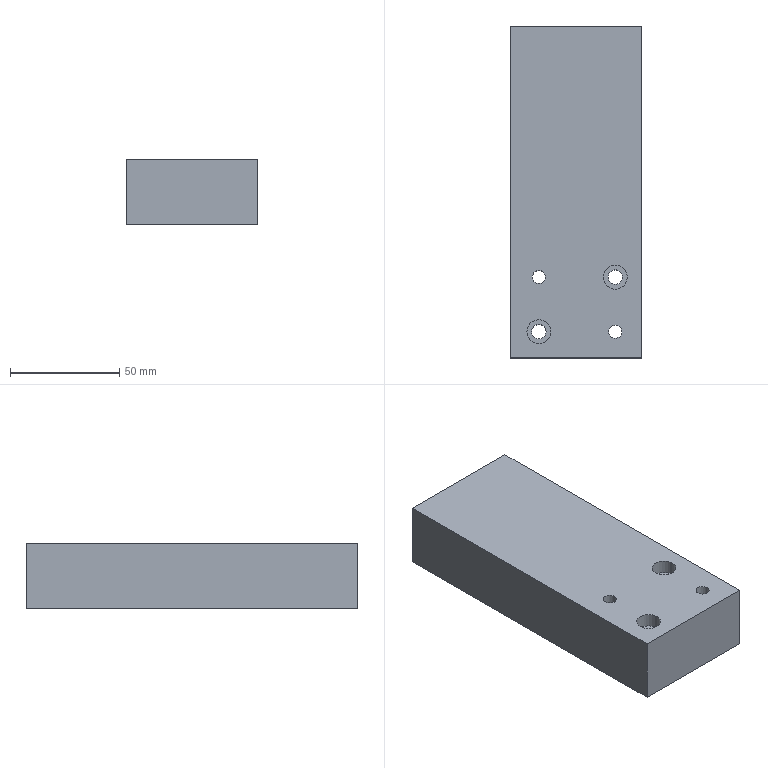Part | NX | features BREP 1 | 1 solid | 22 faces | box 60 x 152 x 30 mm | volume 267751 mm3 | cylinder 10 | plane 8 | cone 4 | commonest cylinder face diameters 6 x4 5 x2 6.6 x2 11 x2
STEP:
#1=CARTESIAN_POINT('',(30.,-76.,0.));
#2=VERTEX_POINT('',#1);
#3=CARTESIAN_POINT('',(30.,76.,0.));
#4=VERTEX_POINT('',#3);
#5=CARTESIAN_POINT('',(30.,76.,0.));
#6=DIRECTION('',(0.,1.,0.));
#7=VECTOR('',#6,1000.);
#8=LINE('',#5,#7);
#9=EDGE_CURVE('',#2,#4,#8,.T.);
#10=ORIENTED_EDGE('',*,*,#9,.T.);
#11=CARTESIAN_POINT('',(30.,76.,30.));
#12=VERTEX_POINT('',#11);
#13=CARTESIAN_POINT('',(30.,76.,30.));
#14=DIRECTION('',(0.,0.,-1.));
#15=VECTOR('',#14,1000.);
#16=LINE('',#13,#15);
#17=EDGE_CURVE('',#12,#4,#16,.T.);
#18=ORIENTED_EDGE('',*,*,#17,.F.);
#19=CARTESIAN_POINT('',(30.,-76.,30.));
#20=VERTEX_POINT('',#19);
#21=CARTESIAN_POINT('',(30.,76.,30.));
#22=DIRECTION('',(0.,1.,0.));
#23=VECTOR('',#22,1000.);
#24=LINE('',#21,#23);
#25=EDGE_CURVE('',#20,#12,#24,.T.);
#26=ORIENTED_EDGE('',*,*,#25,.F.);
#27=CARTESIAN_POINT('',(30.,-76.,30.));
#28=DIRECTION('',(0.,0.,-1.));
#29=VECTOR('',#28,1000.);
#30=LINE('',#27,#29);
#31=EDGE_CURVE('',#20,#2,#30,.T.);
#32=ORIENTED_EDGE('',*,*,#31,.T.);
#33=EDGE_LOOP('',(#10,#18,#26,#32));
#34=FACE_BOUND('',#33,.T.);
#35=CARTESIAN_POINT('',(30.,76.,30.));
#36=DIRECTION('',(-1.,0.,0.));
#37=DIRECTION('',(0.,1.,0.));
#38=AXIS2_PLACEMENT_3D('',#35,#36,#37);
#39=PLANE('',#38);
#40=ADVANCED_FACE('',(#34),#39,.F.);
#41=CARTESIAN_POINT('',(-10.,76.,17.5));
#42=VERTEX_POINT('',#41);
#43=CARTESIAN_POINT('',(-10.,76.,15.));
#44=DIRECTION('',(0.,1.,0.));
#45=DIRECTION('',(0.,0.,1.));
#46=AXIS2_PLACEMENT_3D('',#43,#44,#45);
#47=CIRCLE('',#46,2.5);
#48=EDGE_CURVE('',#42,#42,#47,.T.);
#49=ORIENTED_EDGE('',*,*,#48,.F.);
#50=EDGE_LOOP('',(#49));
#51=FACE_BOUND('',#50,.T.);
#52=CARTESIAN_POINT('',(10.,76.,17.5));
#53=VERTEX_POINT('',#52);
#54=CARTESIAN_POINT('',(10.,76.,15.));
#55=DIRECTION('',(0.,1.,0.));
#56=DIRECTION('',(0.,0.,1.));
#57=AXIS2_PLACEMENT_3D('',#54,#55,#56);
#58=CIRCLE('',#57,2.5);
#59=EDGE_CURVE('',#53,#53,#58,.T.);
#60=ORIENTED_EDGE('',*,*,#59,.F.);
#61=EDGE_LOOP('',(#60));
#62=FACE_BOUND('',#61,.T.);
#63=CARTESIAN_POINT('',(-23.,76.,18.));
#64=VERTEX_POINT('',#63);
#65=CARTESIAN_POINT('',(-23.,76.,15.));
#66=DIRECTION('',(0.,1.,0.));
#67=DIRECTION('',(0.,0.,1.));
#68=AXIS2_PLACEMENT_3D('',#65,#66,#67);
#69=CIRCLE('',#68,3.);
#70=EDGE_CURVE('',#64,#64,#69,.T.);
#71=ORIENTED_EDGE('',*,*,#70,.F.);
#72=EDGE_LOOP('',(#71));
#73=FACE_BOUND('',#72,.T.);
#74=CARTESIAN_POINT('',(23.,76.,18.));
#75=VERTEX_POINT('',#74);
#76=CARTESIAN_POINT('',(23.,76.,15.));
#77=DIRECTION('',(0.,1.,0.));
#78=DIRECTION('',(0.,0.,1.));
#79=AXIS2_PLACEMENT_3D('',#76,#77,#78);
#80=CIRCLE('',#79,3.);
#81=EDGE_CURVE('',#75,#75,#80,.T.);
#82=ORIENTED_EDGE('',*,*,#81,.F.);
#83=EDGE_LOOP('',(#82));
#84=FACE_BOUND('',#83,.T.);
#85=CARTESIAN_POINT('',(-30.,76.,0.));
#86=VERTEX_POINT('',#85);
#87=CARTESIAN_POINT('',(-30.,76.,0.));
#88=DIRECTION('',(-1.,0.,0.));
#89=VECTOR('',#88,1000.);
#90=LINE('',#87,#89);
#91=EDGE_CURVE('',#4,#86,#90,.T.);
#92=ORIENTED_EDGE('',*,*,#91,.T.);
#93=CARTESIAN_POINT('',(-30.,76.,30.));
#94=VERTEX_POINT('',#93);
#95=CARTESIAN_POINT('',(-30.,76.,30.));
#96=DIRECTION('',(0.,0.,-1.));
#97=VECTOR('',#96,1000.);
#98=LINE('',#95,#97);
#99=EDGE_CURVE('',#94,#86,#98,.T.);
#100=ORIENTED_EDGE('',*,*,#99,.F.);
#101=CARTESIAN_POINT('',(-30.,76.,30.));
#102=DIRECTION('',(-1.,0.,0.));
#103=VECTOR('',#102,1000.);
#104=LINE('',#101,#103);
#105=EDGE_CURVE('',#12,#94,#104,.T.);
#106=ORIENTED_EDGE('',*,*,#105,.F.);
#107=ORIENTED_EDGE('',*,*,#17,.T.);
#108=EDGE_LOOP('',(#92,#100,#106,#107));
#109=FACE_BOUND('',#108,.T.);
#110=CARTESIAN_POINT('',(-30.,76.,30.));
#111=DIRECTION('',(0.,-1.,0.));
#112=DIRECTION('',(0.,0.,1.));
#113=AXIS2_PLACEMENT_3D('',#110,#111,#112);
#114=PLANE('',#113);
#115=ADVANCED_FACE('',(#51,#62,#73,#84,#109),#114,.F.);
#116=CARTESIAN_POINT('',(-30.,-76.,0.));
#117=VERTEX_POINT('',#116);
#118=CARTESIAN_POINT('',(-30.,76.,0.));
#119=DIRECTION('',(0.,-1.,0.));
#120=VECTOR('',#119,1000.);
#121=LINE('',#118,#120);
#122=EDGE_CURVE('',#86,#117,#121,.T.);
#123=ORIENTED_EDGE('',*,*,#122,.T.);
#124=CARTESIAN_POINT('',(-30.,-76.,30.));
#125=VERTEX_POINT('',#124);
#126=CARTESIAN_POINT('',(-30.,-76.,30.));
#127=DIRECTION('',(0.,0.,-1.));
#128=VECTOR('',#127,1000.);
#129=LINE('',#126,#128);
#130=EDGE_CURVE('',#125,#117,#129,.T.);
#131=ORIENTED_EDGE('',*,*,#130,.F.);
#132=CARTESIAN_POINT('',(-30.,76.,30.));
#133=DIRECTION('',(0.,-1.,0.));
#134=VECTOR('',#133,1000.);
#135=LINE('',#132,#134);
#136=EDGE_CURVE('',#94,#125,#135,.T.);
#137=ORIENTED_EDGE('',*,*,#136,.F.);
#138=ORIENTED_EDGE('',*,*,#99,.T.);
#139=EDGE_LOOP('',(#123,#131,#137,#138));
#140=FACE_BOUND('',#139,.T.);
#141=CARTESIAN_POINT('',(-30.,76.,30.));
#142=DIRECTION('',(1.,0.,0.));
#143=DIRECTION('',(0.,-1.,0.));
#144=AXIS2_PLACEMENT_3D('',#141,#142,#143);
#145=PLANE('',#144);
#146=ADVANCED_FACE('',(#140),#145,.F.);
#147=CARTESIAN_POINT('',(-30.,-76.,0.));
#148=DIRECTION('',(1.,0.,0.));
#149=VECTOR('',#148,1000.);
#150=LINE('',#147,#149);
#151=EDGE_CURVE('',#117,#2,#150,.T.);
#152=ORIENTED_EDGE('',*,*,#151,.T.);
#153=ORIENTED_EDGE('',*,*,#31,.F.);
#154=CARTESIAN_POINT('',(-30.,-76.,30.));
#155=DIRECTION('',(1.,0.,0.));
#156=VECTOR('',#155,1000.);
#157=LINE('',#154,#156);
#158=EDGE_CURVE('',#125,#20,#157,.T.);
#159=ORIENTED_EDGE('',*,*,#158,.F.);
#160=ORIENTED_EDGE('',*,*,#130,.T.);
#161=EDGE_LOOP('',(#152,#153,#159,#160));
#162=FACE_BOUND('',#161,.T.);
#163=CARTESIAN_POINT('',(-30.,-76.,30.));
#164=DIRECTION('',(0.,1.,0.));
#165=DIRECTION('',(0.,0.,-1.));
#166=AXIS2_PLACEMENT_3D('',#163,#164,#165);
#167=PLANE('',#166);
#168=ADVANCED_FACE('',(#162),#167,.F.);
#169=CARTESIAN_POINT('',(-11.5,-64.,30.));
#170=VERTEX_POINT('',#169);
#171=CARTESIAN_POINT('',(-17.,-64.,30.));
#172=DIRECTION('',(0.,0.,1.));
#173=DIRECTION('',(1.,0.,0.));
#174=AXIS2_PLACEMENT_3D('',#171,#172,#173);
#175=CIRCLE('',#174,5.5);
#176=EDGE_CURVE('',#170,#170,#175,.T.);
#177=ORIENTED_EDGE('',*,*,#176,.F.);
#178=EDGE_LOOP('',(#177));
#179=FACE_BOUND('',#178,.T.);
#180=CARTESIAN_POINT('',(23.5,-39.,30.));
#181=VERTEX_POINT('',#180);
#182=CARTESIAN_POINT('',(18.,-39.,30.));
#183=DIRECTION('',(0.,0.,1.));
#184=DIRECTION('',(1.,0.,0.));
#185=AXIS2_PLACEMENT_3D('',#182,#183,#184);
#186=CIRCLE('',#185,5.5);
#187=EDGE_CURVE('',#181,#181,#186,.T.);
#188=ORIENTED_EDGE('',*,*,#187,.F.);
#189=EDGE_LOOP('',(#188));
#190=FACE_BOUND('',#189,.T.);
#191=CARTESIAN_POINT('',(-14.,-39.,30.));
#192=VERTEX_POINT('',#191);
#193=CARTESIAN_POINT('',(-17.,-39.,30.));
#194=DIRECTION('',(0.,0.,1.));
#195=DIRECTION('',(1.,0.,0.));
#196=AXIS2_PLACEMENT_3D('',#193,#194,#195);
#197=CIRCLE('',#196,3.);
#198=EDGE_CURVE('',#192,#192,#197,.T.);
#199=ORIENTED_EDGE('',*,*,#198,.F.);
#200=EDGE_LOOP('',(#199));
#201=FACE_BOUND('',#200,.T.);
#202=CARTESIAN_POINT('',(21.,-64.,30.));
#203=VERTEX_POINT('',#202);
#204=CARTESIAN_POINT('',(18.,-64.,30.));
#205=DIRECTION('',(0.,0.,1.));
#206=DIRECTION('',(1.,0.,0.));
#207=AXIS2_PLACEMENT_3D('',#204,#205,#206);
#208=CIRCLE('',#207,3.);
#209=EDGE_CURVE('',#203,#203,#208,.T.);
#210=ORIENTED_EDGE('',*,*,#209,.F.);
#211=EDGE_LOOP('',(#210));
#212=FACE_BOUND('',#211,.T.);
#213=ORIENTED_EDGE('',*,*,#25,.T.);
#214=ORIENTED_EDGE('',*,*,#105,.T.);
#215=ORIENTED_EDGE('',*,*,#136,.T.);
#216=ORIENTED_EDGE('',*,*,#158,.T.);
#217=EDGE_LOOP('',(#213,#214,#215,#216));
#218=FACE_BOUND('',#217,.T.);
#219=CARTESIAN_POINT('',(0.,0.,30.));
#220=DIRECTION('',(0.,0.,1.));
#221=DIRECTION('',(-1.,0.,0.));
#222=AXIS2_PLACEMENT_3D('',#219,#220,#221);
#223=PLANE('',#222);
#224=ADVANCED_FACE('',(#179,#190,#201,#212,#218),#223,.T.);
#225=CARTESIAN_POINT('',(-13.7,-64.,0.));
#226=VERTEX_POINT('',#225);
#227=CARTESIAN_POINT('',(-17.,-64.,0.));
#228=DIRECTION('',(0.,0.,1.));
#229=DIRECTION('',(1.,0.,0.));
#230=AXIS2_PLACEMENT_3D('',#227,#228,#229);
#231=CIRCLE('',#230,3.3);
#232=EDGE_CURVE('',#226,#226,#231,.T.);
#233=ORIENTED_EDGE('',*,*,#232,.T.);
#234=EDGE_LOOP('',(#233));
#235=FACE_BOUND('',#234,.T.);
#236=CARTESIAN_POINT('',(21.3,-39.,0.));
#237=VERTEX_POINT('',#236);
#238=CARTESIAN_POINT('',(18.,-39.,0.));
#239=DIRECTION('',(0.,0.,1.));
#240=DIRECTION('',(1.,0.,0.));
#241=AXIS2_PLACEMENT_3D('',#238,#239,#240);
#242=CIRCLE('',#241,3.3);
#243=EDGE_CURVE('',#237,#237,#242,.T.);
#244=ORIENTED_EDGE('',*,*,#243,.T.);
#245=EDGE_LOOP('',(#244));
#246=FACE_BOUND('',#245,.T.);
#247=CARTESIAN_POINT('',(-14.,-39.,0.));
#248=VERTEX_POINT('',#247);
#249=CARTESIAN_POINT('',(-17.,-39.,0.));
#250=DIRECTION('',(0.,0.,1.));
#251=DIRECTION('',(1.,0.,0.));
#252=AXIS2_PLACEMENT_3D('',#249,#250,#251);
#253=CIRCLE('',#252,3.);
#254=EDGE_CURVE('',#248,#248,#253,.T.);
#255=ORIENTED_EDGE('',*,*,#254,.T.);
#256=EDGE_LOOP('',(#255));
#257=FACE_BOUND('',#256,.T.);
#258=CARTESIAN_POINT('',(21.,-64.,0.));
#259=VERTEX_POINT('',#258);
#260=CARTESIAN_POINT('',(18.,-64.,0.));
#261=DIRECTION('',(0.,0.,1.));
#262=DIRECTION('',(1.,0.,0.));
#263=AXIS2_PLACEMENT_3D('',#260,#261,#262);
#264=CIRCLE('',#263,3.);
#265=EDGE_CURVE('',#259,#259,#264,.T.);
#266=ORIENTED_EDGE('',*,*,#265,.T.);
#267=EDGE_LOOP('',(#266));
#268=FACE_BOUND('',#267,.T.);
#269=ORIENTED_EDGE('',*,*,#9,.F.);
#270=ORIENTED_EDGE('',*,*,#151,.F.);
#271=ORIENTED_EDGE('',*,*,#122,.F.);
#272=ORIENTED_EDGE('',*,*,#91,.F.);
#273=EDGE_LOOP('',(#269,#270,#271,#272));
#274=FACE_BOUND('',#273,.T.);
#275=CARTESIAN_POINT('',(0.,0.,0.));
#276=DIRECTION('',(0.,0.,1.));
#277=DIRECTION('',(-1.,0.,0.));
#278=AXIS2_PLACEMENT_3D('',#275,#276,#277);
#279=PLANE('',#278);
#280=ADVANCED_FACE('',(#235,#246,#257,#268,#274),#279,.F.);
#281=ORIENTED_EDGE('',*,*,#265,.F.);
#282=EDGE_LOOP('',(#281));
#283=FACE_BOUND('',#282,.T.);
#284=ORIENTED_EDGE('',*,*,#209,.T.);
#285=EDGE_LOOP('',(#284));
#286=FACE_BOUND('',#285,.T.);
#287=CARTESIAN_POINT('',(18.,-64.,30.));
#288=DIRECTION('',(0.,0.,1.));
#289=DIRECTION('',(-1.,0.,0.));
#290=AXIS2_PLACEMENT_3D('',#287,#288,#289);
#291=CYLINDRICAL_SURFACE('',#290,3.);
#292=ADVANCED_FACE('',(#283,#286),#291,.F.);
#293=ORIENTED_EDGE('',*,*,#254,.F.);
#294=EDGE_LOOP('',(#293));
#295=FACE_BOUND('',#294,.T.);
#296=ORIENTED_EDGE('',*,*,#198,.T.);
#297=EDGE_LOOP('',(#296));
#298=FACE_BOUND('',#297,.T.);
#299=CARTESIAN_POINT('',(-17.,-39.,30.));
#300=DIRECTION('',(0.,0.,1.));
#301=DIRECTION('',(-1.,0.,0.));
#302=AXIS2_PLACEMENT_3D('',#299,#300,#301);
#303=CYLINDRICAL_SURFACE('',#302,3.);
#304=ADVANCED_FACE('',(#295,#298),#303,.F.);
#305=ORIENTED_EDGE('',*,*,#243,.F.);
#306=EDGE_LOOP('',(#305));
#307=FACE_BOUND('',#306,.T.);
#308=CARTESIAN_POINT('',(21.3,-39.,23.6));
#309=VERTEX_POINT('',#308);
#310=CARTESIAN_POINT('',(18.,-39.,23.6));
#311=DIRECTION('',(0.,0.,1.));
#312=DIRECTION('',(1.,0.,0.));
#313=AXIS2_PLACEMENT_3D('',#310,#311,#312);
#314=CIRCLE('',#313,3.3);
#315=EDGE_CURVE('',#309,#309,#314,.T.);
#316=ORIENTED_EDGE('',*,*,#315,.T.);
#317=EDGE_LOOP('',(#316));
#318=FACE_BOUND('',#317,.T.);
#319=CARTESIAN_POINT('',(18.,-39.,30.));
#320=DIRECTION('',(0.,0.,1.));
#321=DIRECTION('',(-1.,0.,0.));
#322=AXIS2_PLACEMENT_3D('',#319,#320,#321);
#323=CYLINDRICAL_SURFACE('',#322,3.3);
#324=ADVANCED_FACE('',(#307,#318),#323,.F.);
#325=ORIENTED_EDGE('',*,*,#315,.F.);
#326=EDGE_LOOP('',(#325));
#327=FACE_BOUND('',#326,.T.);
#328=CARTESIAN_POINT('',(23.5,-39.,23.6));
#329=VERTEX_POINT('',#328);
#330=CARTESIAN_POINT('',(18.,-39.,23.6));
#331=DIRECTION('',(0.,0.,1.));
#332=DIRECTION('',(1.,0.,0.));
#333=AXIS2_PLACEMENT_3D('',#330,#331,#332);
#334=CIRCLE('',#333,5.5);
#335=EDGE_CURVE('',#329,#329,#334,.T.);
#336=ORIENTED_EDGE('',*,*,#335,.T.);
#337=EDGE_LOOP('',(#336));
#338=FACE_BOUND('',#337,.T.);
#339=CARTESIAN_POINT('',(21.3,-39.,23.6));
#340=DIRECTION('',(0.,0.,-1.));
#341=DIRECTION('',(1.,0.,0.));
#342=AXIS2_PLACEMENT_3D('',#339,#340,#341);
#343=PLANE('',#342);
#344=ADVANCED_FACE('',(#327,#338),#343,.F.);
#345=ORIENTED_EDGE('',*,*,#335,.F.);
#346=EDGE_LOOP('',(#345));
#347=FACE_BOUND('',#346,.T.);
#348=ORIENTED_EDGE('',*,*,#187,.T.);
#349=EDGE_LOOP('',(#348));
#350=FACE_BOUND('',#349,.T.);
#351=CARTESIAN_POINT('',(18.,-39.,30.));
#352=DIRECTION('',(0.,0.,1.));
#353=DIRECTION('',(-1.,0.,0.));
#354=AXIS2_PLACEMENT_3D('',#351,#352,#353);
#355=CYLINDRICAL_SURFACE('',#354,5.5);
#356=ADVANCED_FACE('',(#347,#350),#355,.F.);
#357=ORIENTED_EDGE('',*,*,#232,.F.);
#358=EDGE_LOOP('',(#357));
#359=FACE_BOUND('',#358,.T.);
#360=CARTESIAN_POINT('',(-13.7,-64.,23.6));
#361=VERTEX_POINT('',#360);
#362=CARTESIAN_POINT('',(-17.,-64.,23.6));
#363=DIRECTION('',(0.,0.,1.));
#364=DIRECTION('',(1.,0.,0.));
#365=AXIS2_PLACEMENT_3D('',#362,#363,#364);
#366=CIRCLE('',#365,3.3);
#367=EDGE_CURVE('',#361,#361,#366,.T.);
#368=ORIENTED_EDGE('',*,*,#367,.T.);
#369=EDGE_LOOP('',(#368));
#370=FACE_BOUND('',#369,.T.);
#371=CARTESIAN_POINT('',(-17.,-64.,30.));
#372=DIRECTION('',(0.,0.,1.));
#373=DIRECTION('',(-1.,0.,0.));
#374=AXIS2_PLACEMENT_3D('',#371,#372,#373);
#375=CYLINDRICAL_SURFACE('',#374,3.3);
#376=ADVANCED_FACE('',(#359,#370),#375,.F.);
#377=ORIENTED_EDGE('',*,*,#367,.F.);
#378=EDGE_LOOP('',(#377));
#379=FACE_BOUND('',#378,.T.);
#380=CARTESIAN_POINT('',(-11.5,-64.,23.6));
#381=VERTEX_POINT('',#380);
#382=CARTESIAN_POINT('',(-17.,-64.,23.6));
#383=DIRECTION('',(0.,0.,1.));
#384=DIRECTION('',(1.,0.,0.));
#385=AXIS2_PLACEMENT_3D('',#382,#383,#384);
#386=CIRCLE('',#385,5.5);
#387=EDGE_CURVE('',#381,#381,#386,.T.);
#388=ORIENTED_EDGE('',*,*,#387,.T.);
#389=EDGE_LOOP('',(#388));
#390=FACE_BOUND('',#389,.T.);
#391=CARTESIAN_POINT('',(-13.7,-64.,23.6));
#392=DIRECTION('',(0.,0.,-1.));
#393=DIRECTION('',(1.,0.,0.));
#394=AXIS2_PLACEMENT_3D('',#391,#392,#393);
#395=PLANE('',#394);
#396=ADVANCED_FACE('',(#379,#390),#395,.F.);
#397=ORIENTED_EDGE('',*,*,#387,.F.);
#398=EDGE_LOOP('',(#397));
#399=FACE_BOUND('',#398,.T.);
#400=ORIENTED_EDGE('',*,*,#176,.T.);
#401=EDGE_LOOP('',(#400));
#402=FACE_BOUND('',#401,.T.);
#403=CARTESIAN_POINT('',(-17.,-64.,30.));
#404=DIRECTION('',(0.,0.,1.));
#405=DIRECTION('',(-1.,0.,0.));
#406=AXIS2_PLACEMENT_3D('',#403,#404,#405);
#407=CYLINDRICAL_SURFACE('',#406,5.5);
#408=ADVANCED_FACE('',(#399,#402),#407,.F.);
#409=CARTESIAN_POINT('',(23.,62.197,15.));
#410=VERTEX_POINT('',#409);
#411=VERTEX_LOOP('',#410);
#412=FACE_BOUND('',#411,.T.);
#413=CARTESIAN_POINT('',(23.,64.,18.));
#414=VERTEX_POINT('',#413);
#415=CARTESIAN_POINT('',(23.,64.,15.));
#416=DIRECTION('',(0.,1.,0.));
#417=DIRECTION('',(0.,0.,1.));
#418=AXIS2_PLACEMENT_3D('',#415,#416,#417);
#419=CIRCLE('',#418,3.);
#420=EDGE_CURVE('',#414,#414,#419,.T.);
#421=ORIENTED_EDGE('',*,*,#420,.T.);
#422=EDGE_LOOP('',(#421));
#423=FACE_BOUND('',#422,.T.);
#424=CARTESIAN_POINT('',(23.,64.,15.));
#425=DIRECTION('',(0.,1.,0.));
#426=DIRECTION('',(0.,0.,-1.));
#427=AXIS2_PLACEMENT_3D('',#424,#425,#426);
#428=CONICAL_SURFACE('',#427,3.,1.03);
#429=ADVANCED_FACE('',(#412,#423),#428,.F.);
#430=ORIENTED_EDGE('',*,*,#420,.F.);
#431=EDGE_LOOP('',(#430));
#432=FACE_BOUND('',#431,.T.);
#433=ORIENTED_EDGE('',*,*,#81,.T.);
#434=EDGE_LOOP('',(#433));
#435=FACE_BOUND('',#434,.T.);
#436=CARTESIAN_POINT('',(23.,76.,15.));
#437=DIRECTION('',(0.,1.,0.));
#438=DIRECTION('',(0.,0.,-1.));
#439=AXIS2_PLACEMENT_3D('',#436,#437,#438);
#440=CYLINDRICAL_SURFACE('',#439,3.);
#441=ADVANCED_FACE('',(#432,#435),#440,.F.);
#442=CARTESIAN_POINT('',(-23.,62.197,15.));
#443=VERTEX_POINT('',#442);
#444=VERTEX_LOOP('',#443);
#445=FACE_BOUND('',#444,.T.);
#446=CARTESIAN_POINT('',(-23.,64.,18.));
#447=VERTEX_POINT('',#446);
#448=CARTESIAN_POINT('',(-23.,64.,15.));
#449=DIRECTION('',(0.,1.,0.));
#450=DIRECTION('',(0.,0.,1.));
#451=AXIS2_PLACEMENT_3D('',#448,#449,#450);
#452=CIRCLE('',#451,3.);
#453=EDGE_CURVE('',#447,#447,#452,.T.);
#454=ORIENTED_EDGE('',*,*,#453,.T.);
#455=EDGE_LOOP('',(#454));
#456=FACE_BOUND('',#455,.T.);
#457=CARTESIAN_POINT('',(-23.,64.,15.));
#458=DIRECTION('',(0.,1.,0.));
#459=DIRECTION('',(0.,0.,-1.));
#460=AXIS2_PLACEMENT_3D('',#457,#458,#459);
#461=CONICAL_SURFACE('',#460,3.,1.03);
#462=ADVANCED_FACE('',(#445,#456),#461,.F.);
#463=ORIENTED_EDGE('',*,*,#453,.F.);
#464=EDGE_LOOP('',(#463));
#465=FACE_BOUND('',#464,.T.);
#466=ORIENTED_EDGE('',*,*,#70,.T.);
#467=EDGE_LOOP('',(#466));
#468=FACE_BOUND('',#467,.T.);
#469=CARTESIAN_POINT('',(-23.,76.,15.));
#470=DIRECTION('',(0.,1.,0.));
#471=DIRECTION('',(0.,0.,-1.));
#472=AXIS2_PLACEMENT_3D('',#469,#470,#471);
#473=CYLINDRICAL_SURFACE('',#472,3.);
#474=ADVANCED_FACE('',(#465,#468),#473,.F.);
#475=CARTESIAN_POINT('',(10.,59.498,15.));
#476=VERTEX_POINT('',#475);
#477=VERTEX_LOOP('',#476);
#478=FACE_BOUND('',#477,.T.);
#479=CARTESIAN_POINT('',(10.,61.,17.5));
#480=VERTEX_POINT('',#479);
#481=CARTESIAN_POINT('',(10.,61.,15.));
#482=DIRECTION('',(0.,1.,0.));
#483=DIRECTION('',(0.,0.,1.));
#484=AXIS2_PLACEMENT_3D('',#481,#482,#483);
#485=CIRCLE('',#484,2.5);
#486=EDGE_CURVE('',#480,#480,#485,.T.);
#487=ORIENTED_EDGE('',*,*,#486,.T.);
#488=EDGE_LOOP('',(#487));
#489=FACE_BOUND('',#488,.T.);
#490=CARTESIAN_POINT('',(10.,61.,15.));
#491=DIRECTION('',(0.,1.,0.));
#492=DIRECTION('',(0.,0.,-1.));
#493=AXIS2_PLACEMENT_3D('',#490,#491,#492);
#494=CONICAL_SURFACE('',#493,2.5,1.03);
#495=ADVANCED_FACE('',(#478,#489),#494,.F.);
#496=ORIENTED_EDGE('',*,*,#486,.F.);
#497=EDGE_LOOP('',(#496));
#498=FACE_BOUND('',#497,.T.);
#499=ORIENTED_EDGE('',*,*,#59,.T.);
#500=EDGE_LOOP('',(#499));
#501=FACE_BOUND('',#500,.T.);
#502=CARTESIAN_POINT('',(10.,76.,15.));
#503=DIRECTION('',(0.,1.,0.));
#504=DIRECTION('',(0.,0.,-1.));
#505=AXIS2_PLACEMENT_3D('',#502,#503,#504);
#506=CYLINDRICAL_SURFACE('',#505,2.5);
#507=ADVANCED_FACE('',(#498,#501),#506,.F.);
#508=CARTESIAN_POINT('',(-10.,59.498,15.));
#509=VERTEX_POINT('',#508);
#510=VERTEX_LOOP('',#509);
#511=FACE_BOUND('',#510,.T.);
#512=CARTESIAN_POINT('',(-10.,61.,17.5));
#513=VERTEX_POINT('',#512);
#514=CARTESIAN_POINT('',(-10.,61.,15.));
#515=DIRECTION('',(0.,1.,0.));
#516=DIRECTION('',(0.,0.,1.));
#517=AXIS2_PLACEMENT_3D('',#514,#515,#516);
#518=CIRCLE('',#517,2.5);
#519=EDGE_CURVE('',#513,#513,#518,.T.);
#520=ORIENTED_EDGE('',*,*,#519,.T.);
#521=EDGE_LOOP('',(#520));
#522=FACE_BOUND('',#521,.T.);
#523=CARTESIAN_POINT('',(-10.,61.,15.));
#524=DIRECTION('',(0.,1.,0.));
#525=DIRECTION('',(0.,0.,-1.));
#526=AXIS2_PLACEMENT_3D('',#523,#524,#525);
#527=CONICAL_SURFACE('',#526,2.5,1.03);
#528=ADVANCED_FACE('',(#511,#522),#527,.F.);
#529=ORIENTED_EDGE('',*,*,#519,.F.);
#530=EDGE_LOOP('',(#529));
#531=FACE_BOUND('',#530,.T.);
#532=ORIENTED_EDGE('',*,*,#48,.T.);
#533=EDGE_LOOP('',(#532));
#534=FACE_BOUND('',#533,.T.);
#535=CARTESIAN_POINT('',(-10.,76.,15.));
#536=DIRECTION('',(0.,1.,0.));
#537=DIRECTION('',(0.,0.,-1.));
#538=AXIS2_PLACEMENT_3D('',#535,#536,#537);
#539=CYLINDRICAL_SURFACE('',#538,2.5);
#540=ADVANCED_FACE('',(#531,#534),#539,.F.);
#541=CLOSED_SHELL('',(#40,#115,#146,#168,#224,#280,#292,#304,#324,#344,#356,#376,#396,#408,#429,#441,#462,#474,#495,#507,#528,#540));
#542=MANIFOLD_SOLID_BREP('',#541);
#543=(LENGTH_UNIT()NAMED_UNIT(*)SI_UNIT(.MILLI.,.METRE.));
#544=UNCERTAINTY_MEASURE_WITH_UNIT(LENGTH_MEASURE(0.00001),#543,'','');
#545=(NAMED_UNIT(*)PLANE_ANGLE_UNIT()SI_UNIT($,.RADIAN.));
#546=(NAMED_UNIT(*)SI_UNIT($,.STERADIAN.)SOLID_ANGLE_UNIT());
#547=(GEOMETRIC_REPRESENTATION_CONTEXT(3)GLOBAL_UNCERTAINTY_ASSIGNED_CONTEXT((#544))GLOBAL_UNIT_ASSIGNED_CONTEXT((#543,#545,#546))REPRESENTATION_CONTEXT('',''));
#548=ADVANCED_BREP_SHAPE_REPRESENTATION('',(#542),#547);